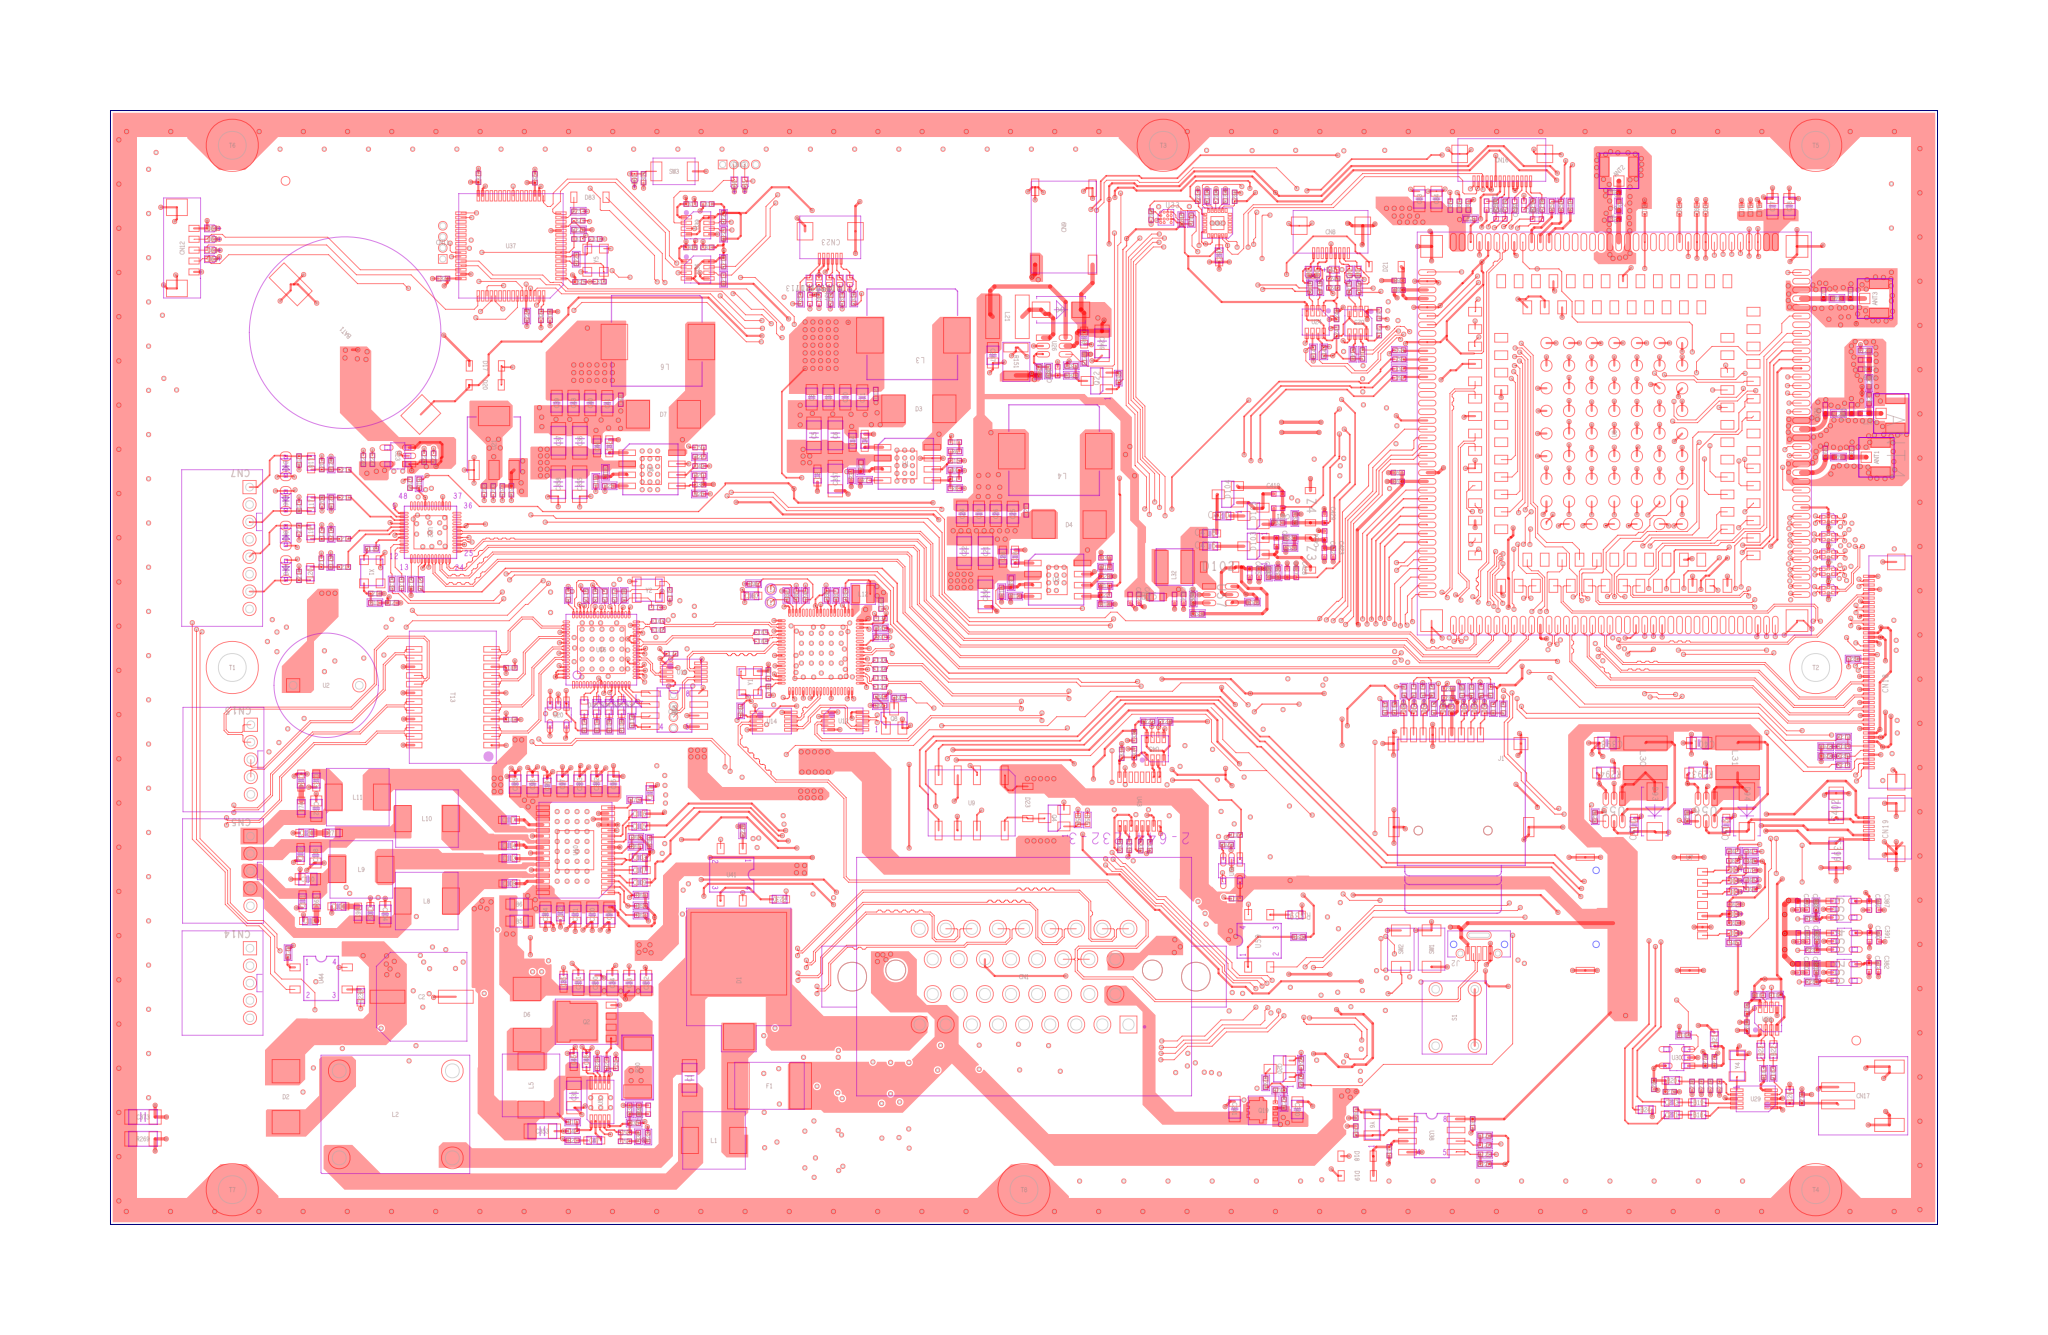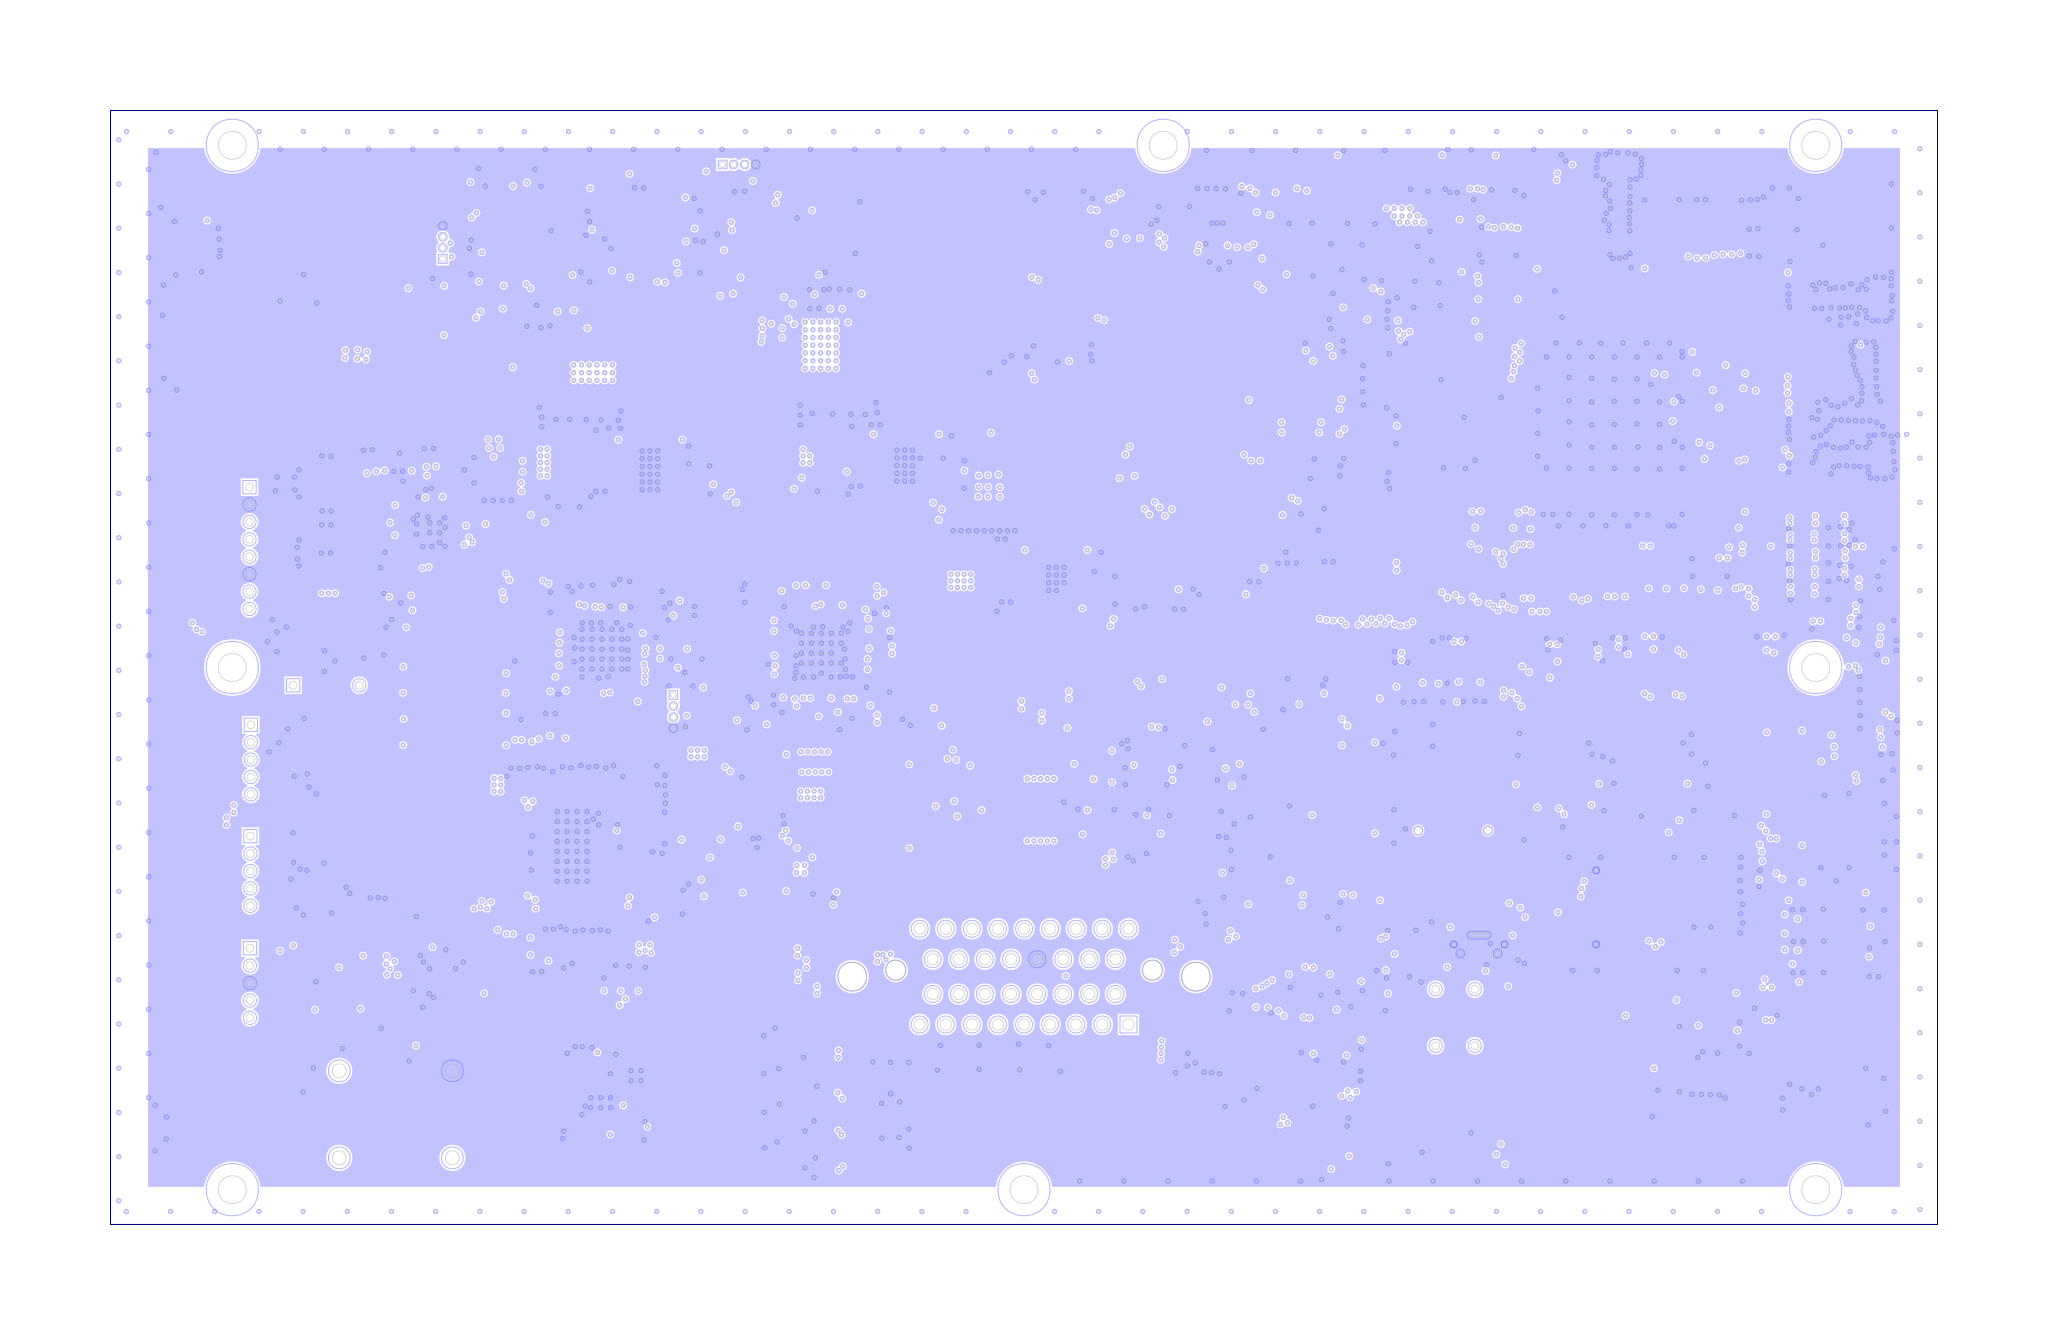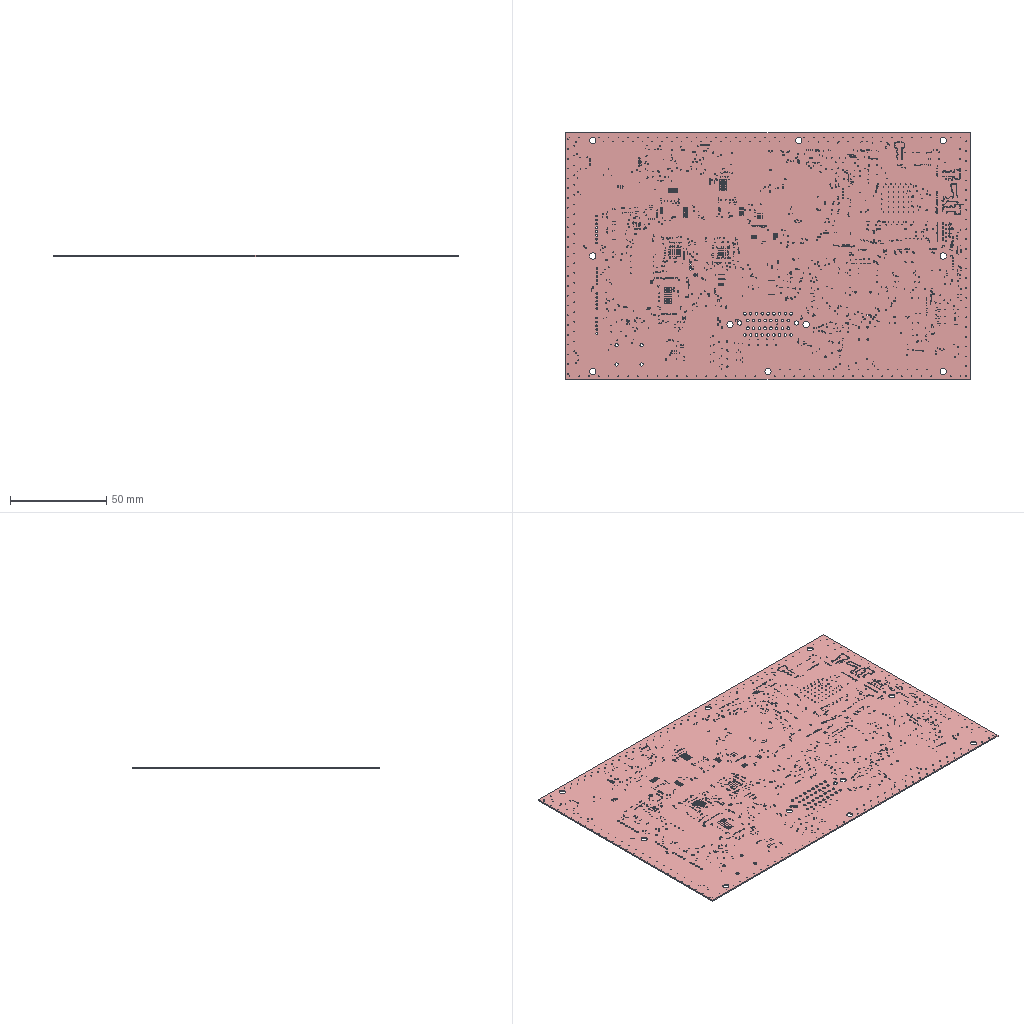Circuit board layout | Cadence Allegro | box 210 x 128 x 0.7 mm
Layer stack:
# Cadence Allegro layer stack of  (unit mm; from the constraint file cross-section; dielectric type: 0 not recorded (Allegro does not mark core vs prepreg), 3 surface material)
index,name,kind,layer,copper_thickness_mm,dielectric_type,dielectric_thickness_mm,dielectric_material,dielectric_constant
0,Top Surface,other,,,,,,
1,TOP,copper,TOP,0.0305,,,,
2,Dielectric1,dielectric,,,0,0.2032,FR-4,4.5
3,L2-GND1,copper,L2-GND1,0.0305,,,,
4,Dielectric2,dielectric,,,0,0.2032,FR-4,4.5
5,L3-PWR,copper,L3-PWR,0.0305,,,,
6,Dielectric3,dielectric,,,0,0.2032,FR-4,4.5
7,BOTTOM,copper,BOTTOM,0.0305,,,,
8,Bottom Surface,other,,,,,,
# drill layer pairs: low layer,high layer
drill_pair,TOP,BOTTOM
Part placement, first 540 of 973 lines:
REFDES,COMP_VALUE,SYM_NAME,SYM_X,SYM_Y,SYM_ROTATE,SYM_MIRROR
ANT1,U.FL-R-SMT-1(80),IPEX,8036.000,5758.000,270.000,NO
ANT2,U.FL-R-SMT-1(80),IPEX,6851.586,7071.978,0.000,NO
ANT3,U.FL-R-SMT-1(80),IPEX,8029.000,6476.000,270.000,NO
ANT4,U.FL-R-SMT-1(80),IPEX,8103.000,5956.000,270.000,NO
B1,120R@100MHz,R0402,6380.000,6896.000,90.000,NO
B2,120R@100MHz,R0402,5858.000,6201.000,180.000,NO
B3,120R@100MHz,R0402,5858.000,6158.000,180.000,NO
B4,120R@100MHz,R0402,5858.000,6117.000,180.000,NO
B5,600R@100MHz,R0805,1875.000,3659.000,0.000,NO
B6,600R@100MHz,R0805,1875.000,3736.000,0.000,NO
B7,120R@100MHz,R0402,2492.000,4867.000,0.000,YES
B8,120R@100MHz,R0402,2474.000,5050.000,0.000,YES
B9,120R@100MHz,R0402,2197.000,5205.000,0.000,YES
B10,120R@100MHz,R0402,2196.000,5113.000,0.000,YES
B11,120R@100MHz,R0402,1223.000,5099.000,180.000,NO
B12,120R@100MHz,R0402,1368.000,5588.000,0.000,YES
B13,120R@100MHz,R0402,1266.000,5652.000,90.000,YES
B14,120R@100MHz,R0402,1518.000,5656.000,90.000,YES
B15,120R@100MHz,R0402,1423.000,5638.000,270.000,NO
B18,1K@100MHz,R0603,7211.000,2783.000,180.000,NO
B19,1K@100MHz,R0603,7212.000,2839.000,180.000,NO
B20,1K@100MHz,R0603,7092.000,2938.000,180.000,NO
B21,1K@100MHz,R0603,7284.000,3125.000,90.000,NO
B22,1K@100MHz,R0603,7551.000,3073.000,270.000,NO
B23,1K@100MHz,R0603,7494.000,3073.000,270.000,NO
B24,1K@100MHz,R0603,6973.000,2806.000,180.000,NO
B25,120R@100MHz,R0603,4760.000,5125.000,0.000,NO
BAT1,BS-08-B2AA008,CR2032,1073.714,6307.425,135.000,NO
C1,10uF,C1206,2646.000,2950.000,90.000,NO
C2,220uF,ED10,1434.000,3317.000,90.000,NO
C3,0.1uF,C0603,3225.000,5675.000,270.000,NO
C4,0.1uF,C0603,3439.000,5832.000,90.000,NO
C5,10uF,C1206,3209.000,5857.000,90.000,NO
C6,10uF,C1206,3306.000,5857.000,90.000,NO
C7,4.7nF,C0402,3846.000,5659.000,180.000,NO
C8,47uF,C0805,3199.000,6029.000,270.000,NO
C9,47uF,C0805,3275.000,6029.000,270.000,NO
C10,47uF,C0805,3351.000,6029.000,270.000,NO
C11,47uF,C0805,3428.000,6028.000,270.000,NO
C12,0.1uF,C0402,3489.000,6044.000,270.000,NO
C14,0.1uF,C0603,3384.000,5832.000,90.000,NO
C15,4.7nF,C0402,3847.000,5742.000,0.000,NO
C17,4.7nF,C0402,3847.000,5826.000,180.000,NO
C18,0.1uF,C0603,4119.000,5308.000,90.000,NO
C19,47uF,C0805,3956.000,5502.000,270.000,NO
C20,22uF,C0805,959.000,4836.000,180.000,YES
C21,10uF,C1206,3986.000,5333.000,90.000,NO
C22,10uF,C1206,3889.000,5333.000,90.000,NO
C23,4.7nF,C0402,4526.000,5135.000,180.000,NO
C24,47uF,C0805,3880.000,5502.000,270.000,NO
C25,47uF,C0805,4109.000,5501.000,270.000,NO
C26,47uF,C0805,4032.000,5502.000,270.000,NO
C27,0.1uF,C0402,4170.000,5517.000,270.000,NO
C28,0.1uF,C0603,4064.000,5308.000,90.000,NO
C29,4.7nF,C0402,4528.000,5219.000,0.000,NO
C30,4.7nF,C0402,4528.000,5303.000,180.000,NO
C31,10uF,C1206,2123.000,2870.000,270.000,NO
C32,0.1uF,C0603,2283.000,5807.000,90.000,NO
C33,22uF,C0805,2373.000,3379.000,90.000,NO
C34,22uF,C0805,2297.000,3379.000,90.000,NO
C35,0.1uF,C0603,2076.000,3385.000,90.000,NO
C36,10uF,C1206,2150.000,5832.000,90.000,NO
C37,10uF,C1206,2053.000,5832.000,90.000,NO
C38,4.7nF,C0402,2690.000,5634.000,180.000,NO
C39,47uF,C0805,2045.000,6003.000,270.000,NO
C40,47uF,C0805,2197.000,6003.000,270.000,NO
C41,47uF,C0805,2274.000,6002.000,270.000,NO
C42,120pF,C0402,2117.000,2709.000,180.000,NO
C43,47uF,C0805,2121.000,6003.000,270.000,NO
C44,0.1uF,C0402,2335.000,6018.000,270.000,NO
C45,0.1uF,C0603,2122.000,3031.000,90.000,NO
C46,0.1uF,C0603,2228.000,5807.000,90.000,NO
C47,220nF,C0603,2215.000,2667.000,0.000,NO
C48,1uF,C0603,2179.000,3031.000,90.000,NO
C49,4.7nF,C0402,2691.000,5718.000,0.000,NO
C50,4.7nF,C0402,2691.000,5802.000,180.000,NO
C51,100pF,C0402,2313.000,3013.000,90.000,NO
C52,22nF,C0402,2354.000,2663.000,0.000,NO
C53,39pF,C0402,2354.000,2703.000,0.000,NO
C60,0.1uF,C0402,6364.000,3432.000,270.000,YES
C61,0.1uF,C0402,5889.000,3372.000,270.000,YES
C62,0.1uF,C0402,7372.000,3735.000,0.000,NO
C63,10uF,C0402,7371.000,3651.000,0.000,NO
C64,33pF,C0402,7447.000,3803.000,0.000,NO
C65,2.2pF(NC),C0402,7905.000,5778.000,90.000,NO
C66,2.2pF(NC),C0402,7786.000,5778.000,90.000,NO
C67,33pF,C0402,7369.000,3932.000,0.000,NO
C68,2.2pF(NC),C0402,6832.071,6956.083,180.000,NO
C69,2.2pF(NC),C0402,6832.071,6835.083,180.000,NO
C70,2.2pF(NC),C0402,7900.000,6496.000,90.000,NO
C71,2.2pF(NC),C0402,7778.000,6495.000,90.000,NO
C72,33pF,C0402,7447.000,3889.000,0.000,NO
C73,0.1uF,C0402,5767.000,3388.000,270.000,YES
C74,33pF,C0402,7407.000,6878.000,90.000,NO
C75,10pF,C0402,7447.000,6878.000,90.000,NO
C76,0.1uF,C0402,7487.000,6878.000,90.000,NO
C77,47uF,C0805,7547.000,6893.000,90.000,NO
C78,47uF,C0805,7623.000,6893.000,90.000,NO
C79,10uF,C0402,6968.000,6878.000,90.000,NO
C80,10uF,C0402,7244.000,6878.000,90.000,NO
C81,10uF,C0402,7204.000,6878.000,90.000,NO
C82,10uF,C0402,7125.000,6878.000,90.000,NO
C83,47uF,C0805,5949.000,6926.000,90.000,NO
C84,47uF,C0805,6026.000,6926.000,90.000,NO
C85,0.1uF,C0402,6089.000,6896.000,90.000,NO
C86,10pF,C0402,6130.000,6896.000,90.000,NO
C87,33pF,C0402,6170.000,6896.000,90.000,NO
C88,10uF,C0402,5855.000,6557.000,180.000,NO
C89,0.1uF,C0402,5855.000,6514.000,180.000,NO
C90,10uF,C0402,5851.000,5648.000,180.000,NO
C91,0.1uF,C0402,5851.000,5688.000,180.000,NO
C95,22uF,C0805,2302.000,4279.000,90.000,NO
C96,22uF,C0805,2283.000,3688.000,270.000,NO
C97,22uF,C0805,2071.000,4279.000,90.000,NO
C98,22uF,C0805,1936.000,4278.000,90.000,NO
C99,0.1uF,C0603,2002.000,4272.000,90.000,NO
C100,22uF,C0805,2206.000,3689.000,270.000,NO
C101,22uF,C0805,2129.000,3689.000,270.000,NO
C102,0.1uF,C0603,2062.000,3694.000,270.000,NO
C103,1uF,C0603,2421.000,3947.000,0.000,NO
C104,680nF,C0805,1269.000,3690.000,90.000,NO
C105,1nF,C0603,1202.000,3696.000,90.000,NO
C106,10nF,C0603,1057.000,3726.000,0.000,NO
C107,1uF,C0603,2421.000,3890.000,180.000,NO
C108,220nF,C0603,1831.000,3829.000,180.000,NO
C109,1uF,C0603,2421.000,3834.000,180.000,NO
C110,680nF,C0805,919.000,3849.000,180.000,NO
C111,1nF,C0603,895.000,3749.000,270.000,NO
C112,10nF,C0603,929.000,3660.000,0.000,NO
C113,220nF,C0603,1831.000,3944.000,180.000,NO
C114,220nF,C0603,1830.000,4001.000,180.000,NO
C115,1uF,C0603,2419.000,4088.000,180.000,NO
C116,1uF,C0603,2420.000,4145.000,180.000,NO
C117,220nF,C0603,1829.000,4117.000,180.000,NO
C118,680nF,C0805,954.000,3957.000,270.000,NO
C119,1nF,C0603,886.000,3963.000,270.000,NO
C120,10nF,C0603,912.000,4058.000,0.000,NO
C121,1uF,C0603,2467.000,4238.000,270.000,NO
C122,680nF,C0805,957.000,4168.000,90.000,NO
C123,1nF,C0603,957.000,4295.000,270.000,NO
C124,10nF,C0603,889.000,4295.000,270.000,NO
C125,22uF,C0805,2463.000,4230.000,180.000,YES
C126,22uF,C0805,2463.000,4318.000,180.000,YES
C127,22uF,C0805,2463.000,4152.000,180.000,YES
C128,1uF,C0603,2347.000,4027.000,0.000,YES
C129,0.1uF,C0402,1515.000,3555.000,90.000,YES
C130,0.1uF,C0402,3362.000,4605.000,180.000,YES
C131,10uF,C0402,3510.000,5028.000,180.000,NO
C132,10uF,C0402,3407.000,5028.000,0.000,YES
C133,0.1uF,C0402,3507.000,4840.000,180.000,NO
C134,0.1uF,C0402,3507.000,4799.000,180.000,NO
C135,0.1uF,C0402,3508.000,4759.000,180.000,NO
C136,0.1uF,C0402,2985.000,4631.000,180.000,YES
C137,0.1uF,C0402,3508.000,4719.000,180.000,NO
C138,18pF,C0402,3003.000,4776.000,90.000,NO
C139,18pF,C0402,3003.000,4701.000,270.000,NO
C140,10uF,C0402,3411.000,4715.000,270.000,YES
C141,10uF,C0402,3329.000,4715.000,270.000,YES
C142,0.1uF,C0402,3513.000,5091.000,270.000,NO
C143,0.1uF,C0402,3402.000,4798.000,0.000,YES
C144,0.1uF,C0402,3287.000,4715.000,270.000,YES
C145,0.1uF,C0402,3161.000,4715.000,270.000,YES
C146,0.1uF,C0402,3086.000,4774.000,180.000,YES
C147,0.1uF,C0402,3086.000,4861.000,180.000,YES
C148,0.1uF,C0402,3086.000,4971.000,180.000,YES
C149,0.1uF,C0402,3086.000,5019.000,180.000,YES
C150,0.1uF,C0402,3249.000,5036.000,90.000,YES
C151,0.1uF,C0402,3402.000,4890.000,0.000,YES
C152,0.1uF,C0402,3370.000,4715.000,270.000,YES
C153,0.1uF,C0402,3402.000,4845.000,0.000,YES
C154,0.1uF,C0402,3208.000,4715.000,270.000,YES
C155,0.1uF,C0402,3114.000,4715.000,270.000,YES
C156,0.1uF,C0402,3086.000,4814.000,180.000,YES
C157,0.1uF,C0402,3207.000,5036.000,90.000,YES
C158,0.1uF,C0402,3407.000,4987.000,0.000,YES
C159,0.1uF,C0402,3351.000,5036.000,90.000,YES
C160,1uF,C0603,2926.000,5131.000,180.000,NO
C161,1nF,C1206,957.000,4414.000,180.000,YES
C162,10uF,C0402,1836.000,4805.000,0.000,NO
C163,0.1uF,C0402,1836.000,4571.000,0.000,NO
C164,1nF,C1206,1158.000,4415.000,0.000,YES
C165,0.1uF,C0402,2970.000,4966.000,0.000,NO
C166,0.1uF,C0402,2505.000,4976.000,0.000,NO
C167,0.1uF,C0402,2504.000,5017.000,0.000,NO
C168,0.1uF,C0402,2970.000,4925.000,0.000,NO
C169,0.1uF,C0402,2685.000,4672.000,0.000,YES
C170,15pF,C0402,2557.000,5138.000,90.000,NO
C171,15pF,C0402,2492.000,5078.000,180.000,NO
C172,0.1uF,C0402,2563.000,4869.000,0.000,NO
C173,0.1uF,C0402,2492.000,4738.000,180.000,YES
C174,10uF,C0402,2079.000,4578.000,270.000,YES
C175,10uF,C0402,2078.000,4658.000,90.000,YES
C176,0.1uF,C0402,2264.000,5028.000,90.000,YES
C177,0.1uF,C0402,2298.000,4738.000,270.000,YES
C178,0.1uF,C0402,2341.000,5028.000,90.000,YES
C179,0.1uF,C0402,2110.000,4918.000,180.000,YES
C180,0.1uF,C0402,2141.000,5028.000,90.000,YES
C181,0.1uF,C0402,2474.000,4966.000,180.000,YES
C182,0.1uF,C0402,2474.000,5007.000,180.000,YES
C183,10uF,C0402,2386.000,4824.000,0.000,YES
C184,0.1uF,C0402,2386.000,4865.000,0.000,YES
C185,10uF,C0402,2386.000,4964.000,0.000,YES
C186,0.1uF,C0402,2386.000,4906.000,0.000,YES
C187,0.1uF,C0402,2386.000,4776.000,0.000,YES
C188,0.1uF,C0402,2257.000,4738.000,270.000,YES
C189,0.1uF,C0402,2223.000,5028.000,90.000,YES
C190,0.1uF,C0402,2110.000,4806.000,180.000,YES
C191,0.1uF,C0402,2182.000,5028.000,90.000,YES
C192,0.1uF,C0402,2110.000,4966.000,180.000,YES
C193,0.1uF,C0402,2110.000,4871.000,180.000,YES
C194,10uF,C0402,2284.000,5163.000,180.000,YES
C195,0.1uF,C0402,2284.000,5205.000,180.000,YES
C196,10uF,C0402,2037.000,5119.000,0.000,YES
C197,0.1uF,C0402,2037.000,5078.000,0.000,YES
C198,10uF,C0402,2622.000,5083.000,180.000,YES
C199,0.1uF,C0402,2622.000,5042.000,180.000,YES
C200,10uF,C0402,2196.000,5155.000,180.000,YES
C201,0.1uF,C0402,2117.000,5120.000,0.000,YES
C202,10uF,C0402,1717.000,5608.000,270.000,NO
C203,0.1uF,C0402,1758.000,5608.000,270.000,NO
C204,10uF,C0402,1840.000,5608.000,270.000,NO
C205,0.1uF,C0402,1799.000,5608.000,270.000,NO
C206,180pF,C0402,879.000,5743.000,270.000,NO
C207,180pF,C0402,982.000,5722.000,90.000,NO
C208,180pF,C0402,879.000,5534.000,90.000,NO
C209,180pF,C0402,983.000,5556.000,270.000,NO
C210,0.1uF,C0402,1084.000,5575.000,0.000,NO
C211,0.1uF,C0402,1084.000,5701.000,0.000,NO
C212,180pF,C0402,879.000,5429.000,270.000,NO
C213,180pF,C0402,982.000,5408.000,90.000,NO
C214,0.1uF,C0402,1082.000,5389.000,0.000,NO
C215,0.1uF,C0402,1082.000,5261.000,0.000,NO
C216,180pF,C0402,879.000,5221.000,90.000,NO
C217,180pF,C0402,980.000,5281.000,90.000,NO
C218,0.1uF,C0402,1223.000,5141.000,0.000,NO
C219,0.1uF,C0402,1300.000,5099.000,0.000,NO
C220,0.1uF,C0402,1368.000,5672.000,0.000,YES
C221,10uF,C0402,1368.000,5630.000,0.000,YES
C222,0.1uF,C0402,1368.000,5546.000,180.000,YES
C223,10uF,C0402,1368.000,5505.000,180.000,YES
C224,0.1uF,C0402,1445.000,5756.000,90.000,NO
C225,10uF,C0402,1488.000,5756.000,90.000,NO
C226,0.1uF,C0402,1170.000,5746.000,90.000,NO
C227,10uF,C0402,1211.000,5746.000,90.000,NO
C228,0.1uF,C0402,1368.000,5410.000,180.000,YES
C229,22uF,C0805,814.000,4924.000,0.000,YES
C230,10uF,C0402,1308.000,5652.000,270.000,YES
C231,22uF,C0805,822.000,5058.000,90.000,YES
C232,0.1uF,C0402,1529.000,5525.000,90.000,YES
C233,0.1uF,C0402,1480.000,5311.000,270.000,YES
C234,0.1uF,C0402,1437.000,5655.000,90.000,YES
C235,10uF,C0402,1478.000,5655.000,90.000,YES
C236,0.1uF,C0402,1580.000,5440.000,0.000,YES
C237,0.1uF,C0402,1580.000,5355.000,0.000,YES
C238,0.1uF,C0402,1450.000,5525.000,90.000,YES
C239,0.1uF,C0402,1439.000,5311.000,270.000,YES
C240,0.1uF,C0402,1381.000,5638.000,90.000,NO
C241,0.1uF,C0402,5574.000,6325.000,90.000,NO
C242,0.1uF,C0402,5574.000,6401.000,270.000,NO
C244,0.1uF,C0402,5559.000,6566.000,180.000,NO
C245,10uF,C0402,5559.000,6524.000,180.000,NO
C247,47uF,C0805,4019.000,6219.000,270.000,NO
C248,1uF,C0603,4432.000,6299.000,270.000,NO
C249,10uF,C1206,4513.000,6273.000,270.000,NO
C268,0.1uF,C0402,7431.000,3260.000,270.000,NO
C269,0.1uF,C0402,7431.000,3182.000,90.000,NO
C270,22pF,C0402,7680.000,2855.000,90.000,NO
C271,1uF,C0603,7091.000,2783.000,180.000,NO
C272,10uF,C0402,7284.000,3025.000,90.000,NO
C273,1uF,C0603,7091.000,2839.000,180.000,NO
C274,0.1uF,C0402,7243.000,3025.000,90.000,NO
C275,0.1uF,C0402,7225.000,2914.000,270.000,NO
C276,10uF,C0402,7183.000,2914.000,270.000,NO
C277,10pF,C0402,7307.000,2914.000,270.000,NO
C278,2.2nF,C0402,7266.000,2914.000,270.000,NO
C279,0.1uF,C0402,7082.000,2887.000,0.000,NO
C280,10uF,C0402,7010.000,2918.000,270.000,NO
C284,10uF,C0402,6080.000,4711.000,0.000,NO
C285,0.1uF,C0402,6080.000,4669.000,0.000,NO
C286,0.1uF,C0402,5113.000,6936.000,90.000,NO
C287,0.1uF,C0402,4946.000,6936.000,90.000,NO
C288,0.1uF,C0402,5029.000,6936.000,90.000,NO
C289,10uF,C0402,4735.000,6851.000,90.000,NO
C290,1uF,C0603,5043.000,6671.000,270.000,NO
C291,10uF,C1206,5149.000,3232.000,270.000,YES
C292,0.1uF,C0603,5229.000,3207.000,270.000,YES
C293,0.1uF,C0402,5541.000,3357.000,90.000,YES
C294,0.1uF,C0402,5542.000,3280.000,270.000,YES
C295,10uF,C1206,5722.000,3236.000,270.000,YES
C296,0.1uF,C0603,5644.000,3211.000,270.000,YES
C297,4.7nF,C0603,4975.000,3048.000,90.000,YES
C298,4.7nF,C0603,5044.000,2901.000,270.000,YES
C299,22uF,C0805,3246.000,2870.000,0.000,YES
C300,22uF,C0805,3597.000,2917.000,90.000,YES
C301,22uF,C0805,3244.000,2709.000,0.000,YES
C302,22uF,C0805,3594.000,2754.000,90.000,YES
C303,22uF,C0805,3245.000,2543.000,0.000,YES
C304,22uF,C0805,3245.000,3062.000,0.000,YES
C305,22uF,C0805,3595.000,2597.000,270.000,YES
C306,22uF,C0805,3597.000,3055.000,90.000,YES
C307,0.1uF,C0402,2727.000,6707.000,180.000,NO
C308,0.1uF,C0402,2650.000,6707.000,0.000,NO
C309,0.1uF,C0402,2438.000,7020.000,270.000,NO
C310,0.1uF,C0402,2727.000,6903.000,180.000,NO
C311,0.1uF,C0402,2651.000,6903.000,0.000,NO
C312,0.1uF,C0402,5813.000,2618.000,270.000,NO
C313,0.1uF,C0402,6190.000,2744.000,270.000,NO
C314,18pF,C0402,2239.000,6552.000,180.000,NO
C315,0.1uF,C0402,5767.000,6328.000,90.000,NO
C316,18pF,C0402,2220.000,6745.000,0.000,NO
C317,0.1uF,C0402,2143.000,6745.000,0.000,NO
C318,100pF,C0402,2914.000,4004.000,180.000,YES
C319,10uF,C0402,2015.000,6397.000,270.000,NO
C320,0.1uF,C0402,1974.000,6397.000,270.000,NO
C321,0.1uF,C0402,2143.000,6828.000,0.000,NO
C322,0.1uF,C0402,1946.414,7019.828,90.000,NO
C323,0.1uF,C0402,1691.000,7022.000,90.000,NO
C324,0.1uF,C0402,1531.000,6566.000,180.000,NO
C325,0.1uF,C0402,2148.000,6551.000,0.000,NO
C326,100pF,C0402,2990.000,4004.000,0.000,YES
C327,10uF,C0402,2953.000,4580.000,0.000,YES
C328,0.1uF,C0402,2953.000,4539.000,0.000,YES
C329,10uF,C0402,1977.000,3370.000,270.000,YES
C330,0.1uF,C0402,1936.000,3370.000,270.000,YES
C331,0.1uF,C0402,4594.000,3999.000,270.000,NO
C332,0.1uF,C0402,4688.000,3998.000,90.000,NO
C333,0.1uF,C0402,4602.000,4416.000,270.000,NO
C334,0.1uF,C0402,4729.000,3998.000,90.000,NO
C335,0.1uF,C0402,4636.000,3999.000,90.000,NO
C336,0.1uF,C0402,4659.000,4496.000,270.000,NO
C337,0.1uF,C0402,4659.000,4419.000,90.000,NO
C338,100pF,C0402,1444.000,3413.000,270.000,YES
C339,100pF,C0402,1444.000,3336.000,90.000,YES
C340,22uF,C0805,5397.000,2807.000,90.000,NO
C341,22uF,C0805,5113.000,2809.000,90.000,NO
C342,0.1uF,C0402,1377.000,3076.000,90.000,YES
C343,0.1uF,C0402,5492.000,4782.000,90.000,YES
C344,0.1uF,C0402,5492.000,4707.000,270.000,YES
C350,22uF,C0805,2220.000,3379.000,90.000,NO
C351,22uF,C0805,2143.000,3380.000,90.000,NO
C352,22uF,C0805,2450.000,3379.000,90.000,NO
C353,10uF,C1206,1980.000,2709.000,0.000,NO
C355,10uF,C1206,2149.000,5636.000,270.000,NO
C356,10uF,C1206,3985.000,5137.000,270.000,NO
C357,10uF,C1206,3306.000,5661.000,270.000,NO
C358,10uF,C1206,2052.000,5636.000,270.000,NO
C361,0.1uF,C0402,1368.000,5457.000,180.000,YES
C362,22uF,C0805,2225.000,4280.000,90.000,NO
C363,22uF,C0805,2149.000,4279.000,90.000,NO
C364,22uF,C0805,1994.000,3689.000,270.000,NO
C365,22uF,C0805,1857.000,4279.000,90.000,NO
C368,10pF,C0402,5661.000,2788.000,90.000,NO
C369,10pF,C0402,5661.000,2712.000,270.000,NO
C370,0.1uF,C0402,5767.000,6405.000,270.000,NO
C371,10uF,C0402,5118.000,3761.000,180.000,NO
C372,10uF,C0402,5118.000,4049.000,180.000,NO
C373,1nF,C1206,173.000,2773.000,180.000,NO
C374,100pF,C0402,2459.000,2806.000,90.000,NO
C375,2.2pF(NC),C0402,7905.000,5975.000,90.000,NO
C376,2.2pF(NC),C0402,7786.000,5975.000,90.000,NO
C377,100pF,C0402,7964.000,5956.000,180.000,NO
C378,0.1uF,C0402,7965.000,6198.000,180.000,NO
C379,1uF,C0402,7965.000,6156.000,180.000,NO
C380,0.1uF,C0402,7662.000,3446.000,270.000,NO
C381,10uF,C0402,7703.000,3446.000,270.000,NO
C382,0.1uF,C0402,8026.000,3450.000,270.000,NO
C383,10uF,C0402,7984.000,3450.000,270.000,NO
C384,0.1uF,C0402,7664.000,3586.000,270.000,NO
C385,10uF,C0402,7705.000,3586.000,270.000,NO
C386,0.1uF,C0402,7985.000,3729.000,270.000,NO
C387,10uF,C0402,8027.000,3729.000,270.000,NO
C388,0.1uF,C0402,7703.000,3730.000,270.000,NO
C389,10uF,C0402,7662.000,3730.000,270.000,NO
C390,0.1uF,C0402,7986.000,3586.000,270.000,NO
C391,10uF,C0402,8029.000,3586.000,270.000,NO
C392,0.1uF,C0402,8092.000,4447.000,180.000,YES
C393,0.1uF,C0402,8092.000,4531.000,180.000,YES
C394,0.1uF,C0402,8087.000,4949.000,180.000,YES
C395,0.1uF,C0402,8087.000,4908.000,180.000,YES
C396,0.1uF,C0402,8087.000,4990.000,180.000,YES
C397,0.1uF,C0402,8092.000,4490.000,180.000,YES
C398,47uF,C0805,6798.000,4465.000,180.000,NO
C399,10uF,C1206,7835.000,3956.000,270.000,NO
C400,1uF,C0603,6921.000,4095.000,90.000,NO
C401,47uF,C0805,7215.000,4465.000,180.000,NO
C402,10uF,C1206,7835.000,4183.000,90.000,NO
C403,1uF,C0603,7338.000,4095.000,90.000,NO
C404,33pF,C0402,6316.000,6836.000,0.000,NO
C405,33pF,C0402,6253.000,6896.000,270.000,NO
C406,33pF,C0402,6481.000,6835.000,0.000,NO
C407,33pF,C0402,6422.000,6897.000,90.000,NO
C408,10uF,C0402,5759.000,6461.000,180.000,YES
C409,0.1uF,C0402,5759.000,6420.000,180.000,YES
C412,0.1uF,C0402,4640.000,5117.000,270.000,NO
C413,10uF,C0402,4679.000,5117.000,270.000,NO
C414,0.1uF,C0402,4841.000,5117.000,270.000,NO
C415,10uF,C0402,4882.000,5117.000,270.000,NO
C416,1uF,C0603,5002.000,5355.000,0.000,NO
C417,0.1uF,C0402,5302.000,5373.000,270.000,NO
C418,1uF,C0603,5002.000,5413.000,0.000,NO
C419,0.1uF,C0402,5310.000,5592.000,0.000,NO
C420,1uF,C0603,5062.000,5492.000,0.000,NO
C421,0.1uF,C0402,5310.000,5527.000,180.000,NO
C422,0.1uF,C0402,5519.000,5326.000,270.000,NO
C423,1uF,C0402,5559.000,5326.000,270.000,NO
C424,1uF,C0402,5520.000,5404.000,90.000,NO
C425,0.1uF,C0402,5181.000,5234.000,270.000,NO
C426,1uF,C0402,5223.000,5234.000,270.000,NO
C427,0.1uF,C0402,5351.000,5234.000,270.000,NO
C428,10uF,C0402,5392.000,5234.000,270.000,NO
C429,1uF,C0402,5520.000,5481.000,270.000,NO
C430,0.1uF,C0402,5131.000,4291.000,270.000,YES
C431,100pF,C0402,5314.000,3950.000,0.000,YES
C432,100pF,C0402,5237.000,3950.000,180.000,YES
C433,100pF,C0402,5284.000,4548.000,0.000,YES
C434,1uF,C0402,4312.000,6147.000,90.000,NO
C435,0.1uF,C0402,5013.000,4482.000,90.000,YES
C436,0.1uF,C0402,3191.000,6472.000,270.000,NO
C437,10uF,C0402,3232.000,6472.000,270.000,NO
CN1,TE_2_6447232_3,TE_2-6447232-3,4160.000,3408.000,180.000,NO
CN5,A2008WR-5P,A2008WR_5P,659.000,3886.000,180.000,NO
CN6,1.27-4P(NC),SIP4_1P27,2573.409,4607.181,270.000,NO
CN7,A2008WR-8P,A2008WR_8P,655.016,5347.000,180.000,NO
CN8,KH-FG0.5-H2.0-9PIN,FPC-9-0P5-2MMH,5549.000,6681.000,180.000,NO
CN9,SM02B-BHSS-1-TB,SM02B,4340.000,6798.000,0.000,NO
CN11,1.27-4P(NC),SIP4_1P27,1529.591,6729.819,90.000,NO
CN12,1.25LT-5P,PH125_5P_SMD_B,404.000,6793.000,270.000,NO
CN13,1.27-4P(NC),SIP4_1P27,2871.000,7082.000,0.000,NO
CN14,A2008WR-5P,A2008WR_5P,657.000,3379.000,180.000,NO
CN15,A2008WR-5P,A2008WR_5P,661.000,4390.000,180.000,NO
CN16,X05A20H14G,FPC-14-0P5-2MMH,6324.000,7006.000,180.000,NO
CN17,PH2.0WT-2P,PH20_2_SMD_B,7961.922,2869.000,270.000,NO
CN18,X05A20H45G,FPC-45-0P5-2MMH,7983.000,4786.000,90.000,NO
CN19,X05A10H06G,FPC-6-0P5-2MMH,7983.000,4078.000,90.000,NO
CN20,X05A20H30G,FPC-30-0P5-2MMH,5652.000,6103.000,270.000,YES
CN23,X05A10H06G,FPC-6-0P5-2MMH,3283.000,6656.000,180.000,NO
CN25,FPC05_10P,FPC-10-0P5-2MMH,5654.000,5516.370,270.000,YES
D1,SM8S33A,DO_218AB,2869.000,3324.000,270.000,NO
D2,MBRS360T3G,SMC,820.000,2865.000,90.000,NO
D3,MBRS360T3G,SMC,3684.000,5977.000,0.000,NO
D4,MBRS360T3G,SMC,4364.000,5453.000,0.000,NO
D5,B5819W,SOD-123,998.000,4924.000,0.000,YES
D6,MBRS360T3G,SMC,1911.000,3237.000,90.000,NO
D7,MBRS360T3G,SMC,2528.000,5952.000,0.000,NO
D8,B5819W,SOD-123,5917.500,3465.000,0.000,YES
D9,TPESD8L3.3CT5G,DFN1006_2L,6404.000,3428.000,0.000,YES
D10,TPESD8L3.3CT5G,DFN1006_2L,5929.000,3368.000,0.000,YES
D11,TPESD8L3.3CT5G,DFN1006_2L,7367.000,3792.000,270.000,NO
D12,TPESD8L3.3CT5G,DFN1006_2L,7366.000,3892.000,270.000,NO
D13,TPESD8L3.3CT5G,DFN1006_2L,7367.000,3692.000,270.000,NO
D14,TPESD8L3.3CT5G,DFN1006_2L,7366.000,3842.000,270.000,NO
D15,TPESD8L3.3CT5G,DFN1006_2L,7367.000,3605.000,270.000,NO
D16,TPESD8L3.3CT5G,DFN1006_2L,5807.000,3368.000,0.000,YES
D17,B5819W,SOD-123,1722.500,6171.000,0.000,NO
D18,B5819W,SOD-123,5667.000,2596.000,0.000,NO
D19,B5819W,SOD-123,5668.000,2507.000,0.000,NO
D20,B5819W,SOD-123,1721.500,6085.000,0.000,NO
D21,B5819W,SOD-123,5794.000,6620.000,0.000,NO
D23,B5819W,SOD-123,4177.000,4196.000,90.000,NO
D26,B5819W,SOD-123,2104.500,3713.000,180.000,YES
D27,B5819W,SOD-123,2035.000,4306.000,180.000,YES
D28,B5819W,SOD-123,2377.000,3881.000,90.000,YES
D29,B5819W,SOD-123,2291.000,3881.000,90.000,YES
D30,B5819W,SOD-123,1654.000,3566.000,0.000,YES
D32,GREEN,D0603,2339.000,4628.000,90.000,NO
D33,YELLOW,D0603,2283.000,4628.000,90.000,NO
D34,RED,D0603,2227.000,4628.000,90.000,NO
D35,GREEN,D0603,2170.000,4627.000,90.000,NO
D36,JEB03CX,SOD-323,819.000,5560.000,270.000,NO
D37,JEB03CX,SOD-323,819.000,5717.000,90.000,NO
D38,JEB03CX,SOD-323,819.000,5403.000,90.000,NO
D39,JEB03CX,SOD-323,820.000,5247.000,270.000,NO
D40,TPESD8L3.3CT5G,DFN1006_2L,5670.000,6595.000,180.000,NO
D41,TPESD8L3.3CT5G,DFN1006_2L,5633.000,6595.000,180.000,NO
D42,TPESD8L3.3CT5G,DFN1006_2L,5559.000,6606.000,90.000,NO
D43,SS34,SMA,4237.000,6425.000,0.000,NO
D44,TPESD8L3.3CT5G,DFN1006_2L,5448.000,6594.000,180.000,NO
D45,TPESD8L3.3CT5G,DFN1006_2L,5486.000,6594.000,180.000,NO
D46,TPESD8L3.3CT5G,DFN1006_2L,5877.000,4616.000,0.000,NO
D47,TPESD8L3.3CT5G,DFN1006_2L,6151.000,4616.000,0.000,NO
D48,TPESD8L3.3CT5G,DFN1006_2L,6056.000,4616.000,0.000,NO
D49,TPESD8L3.3CT5G,DFN1006_2L,6197.000,4616.000,0.000,NO
D50,TPESD8L3.3CT5G,DFN1006_2L,6243.000,4616.000,0.000,NO
D51,TPESD8L3.3CT5G,DFN1006_2L,5925.000,4616.000,0.000,NO
D52,TPESD8L3.3CT5G,DFN1006_2L,5970.000,4616.000,0.000,NO
D53,TPESD8L3.3CT5G,DFN1006_2L,6093.000,4616.000,0.000,NO
D54,MURS260,SMA,5145.000,2898.000,270.000,YES
D55,MURS260,SMA,4846.000,3033.000,90.000,YES
D56,SMAJ12A,SMA,3957.000,3042.000,90.000,YES
D57,SMAJ12A,SMA,4140.000,3042.000,90.000,YES
D58,SMAJ12A,SMA,4324.000,3041.000,90.000,YES
D59,SMAJ12A,SMA,3769.000,3042.000,90.000,YES
D60,TPESD8L3.3CT5G,DFN1006_2L,2397.000,7024.000,180.000,NO
D61,TPESD8L3.3CT5G,DFN1006_2L,479.000,6793.000,270.000,NO
D62,TPESD8L3.3CT5G,DFN1006_2L,479.000,6744.000,270.000,NO
D63,TPESD8L3.3CT5G,DFN1006_2L,479.000,6694.000,270.000,NO
D64,TPESD8L3.3CT5G,DFN1006_2L,479.000,6654.000,270.000,NO
D65,TPESD8L3.3CT5G,DFN1006_2L,2896.000,6998.000,180.000,NO
D66,TPESD8L3.3CT5G,DFN1006_2L,2849.000,6998.000,180.000,NO
D67,PESD2CAN,SOT-23,2952.000,3905.000,0.000,YES
D68,PESD2CAN,SOT-23,953.000,3385.000,270.000,YES
D69,SMAJ12A,SMA,4648.000,4192.000,90.000,YES
D70,SMAJ12A,SMA,4778.000,4191.000,90.000,YES
D73,B5819W,SOD-123,1537.000,3109.000,0.000,YES
D79,TPESD8L3.3CT5G,DFN1006_2L,1598.000,6703.000,270.000,YES
D80,TPESD8L3.3CT5G,DFN1006_2L,1599.000,6740.000,270.000,YES
D83,B5819W,SOD-123,2195.500,6934.000,180.000,NO
D84,B5819W,SOD-123,1537.000,3198.000,0.000,YES
D85,B5819W,SOD-123,1654.000,3653.000,0.000,YES
D86,SMBJ33A,SMB,897.000,3020.000,270.000,YES
D87,SMBJ6.5CA,SMB,2935.000,3745.000,0.000,YES
D88,SMBJ6.5A,SMB,3168.000,3746.000,0.000,YES
D89,SMBJ6.5A,SMB,2702.000,3745.000,180.000,YES
D90,SMBJ6.5CA,SMB,1109.000,3375.000,270.000,YES
D91,SMBJ6.5A,SMB,1306.000,3291.000,0.000,YES
D92,SMBJ6.5A,SMB,1305.000,3459.000,0.000,YES
D93,SS34,SMA,7014.000,4245.000,270.000,NO
D94,SS34,SMA,7431.000,4245.000,270.000,NO
D95,SMBJ33A,SMB,1038.000,3700.000,90.000,YES
D96,TPESD8L3.3CT5G,DFN1006_2L,5755.000,6381.000,270.000,YES
D102,B5819W,SOD-123,5045.000,5261.000,0.000,NO
D103,BAT54S KL4,SOT-23,5198.000,5355.000,90.000,NO
D104,BAT54S KL4,SOT-23,5082.000,5590.000,90.000,NO
D105,BAT54S KL4,SOT-23,5198.000,5492.000,90.000,NO
D106,SMBJ6.5CA,SMB,5260.000,3684.000,0.000,YES
D107,SMBJ6.5A,SMB,5498.000,3683.000,0.000,YES
D108,SMBJ6.5A,SMB,5025.000,3684.000,180.000,YES
D109,PESD2CAN,SOT-23,5269.000,3855.000,0.000,YES
D110,TPESD8L3.3CT5G,DFN1006_2L,3326.000,6554.000,180.000,NO
D111,TPESD8L3.3CT5G,DFN1006_2L,3371.000,6554.000,180.000,NO
D112,TPESD8L3.3CT5G,DFN1006_2L,3278.000,6554.000,180.000,NO
D113,TPESD8L3.3CT5G,DFN1006_2L,3189.000,6554.000,180.000,NO
D114,B5819W,SOD-123,4896.000,4711.000,90.000,YES
D115,SMBJ33A,SMB,4967.000,4099.000,0.000,YES
D116,B5819W,SOD-123,4987.000,4711.000,90.000,YES
D117,TPESD8L3.3CT5G,DFN1006_2L,3232.000,6554.000,180.000,NO
F1,SMD2920P185TS,R2920,3008.000,2914.000,180.000,NO
F2,BSMD0603-001-60V,R0603,4049.000,2892.000,270.000,YES
F3,BSMD0603-001-60V,R0603,4231.000,2892.000,270.000,YES
Pad and via stacks, first 110 of 429 lines:
# Allegro (Cadence) via spans and padstacks; design units: ("mils" 3 1000)
# via spans: padstack,start_layer,end_layer,net_example,count
0503,ETCH/TOP,ETCH/BOTTOM,EGND,2319
# Allegro padstack definitions: name,start_layer,end_layer,drill,plating,holeType,type
PAD1,"ETCH/TOP","ETCH/TOP",0.0,"NON_PLATED","none","smd"
PAD49,"ETCH/TOP","ETCH/TOP",0.0,"NON_PLATED","none","smd"
PAD28,"ETCH/TOP","ETCH/TOP",0.0,"NON_PLATED","none","smd"
PAD16,"ETCH/TOP","ETCH/TOP",0.0,"NON_PLATED","none","smd"
PAD17,"ETCH/TOP","ETCH/TOP",0.0,"NON_PLATED","none","smd"
PAD63,"ETCH/TOP","ETCH/TOP",0.0,"NON_PLATED","none","smd"
PAD76,"ETCH/TOP","ETCH/TOP",0.0,"NON_PLATED","none","smd"
PAD77,"ETCH/TOP","ETCH/TOP",0.0,"NON_PLATED","none","smd"
PAD54,"ETCH/TOP","ETCH/TOP",0.0,"NON_PLATED","none","smd"
PAD53,"ETCH/TOP","ETCH/TOP",0.0,"NON_PLATED","none","smd"
PAD55,"ETCH/TOP","ETCH/TOP",0.0,"NON_PLATED","none","smd"
PAD56,"ETCH/TOP","ETCH/TOP",0.0,"NON_PLATED","none","smd"
PAD57,"ETCH/TOP","ETCH/TOP",0.0,"NON_PLATED","none","smd"
PAD64,"ETCH/TOP","ETCH/TOP",0.0,"NON_PLATED","none","smd"
PAD43,"ETCH/TOP","ETCH/TOP",0.0,"NON_PLATED","none","smd"
PAD71,"ETCH/TOP","ETCH/TOP",0.0,"NON_PLATED","none","smd"
PAD14,"ETCH/TOP","ETCH/TOP",0.0,"NON_PLATED","none","smd"
PAD58,"ETCH/TOP","ETCH/TOP",0.0,"NON_PLATED","none","smd"
PAD59,"ETCH/TOP","ETCH/TOP",0.0,"NON_PLATED","none","smd"
PAD65,"ETCH/TOP","ETCH/TOP",0.0,"NON_PLATED","none","smd"
PAD60,"ETCH/TOP","ETCH/TOP",0.0,"NON_PLATED","none","smd"
PAD61,"ETCH/TOP","ETCH/TOP",0.0,"NON_PLATED","none","smd"
PAD62,"ETCH/TOP","ETCH/TOP",0.0,"NON_PLATED","none","smd"
PAD72,"ETCH/TOP","ETCH/TOP",0.0,"NON_PLATED","none","smd"
PAD66,"ETCH/TOP","ETCH/TOP",0.0,"NON_PLATED","none","smd"
PAD23,"ETCH/TOP","ETCH/TOP",0.0,"NON_PLATED","none","smd"
PAD24,"ETCH/TOP","ETCH/TOP",0.0,"NON_PLATED","none","smd"
PAD25,"ETCH/TOP","ETCH/TOP",0.0,"NON_PLATED","none","smd"
PAD4,"ETCH/TOP","ETCH/TOP",0.0,"NON_PLATED","none","smd"
PAD5,"ETCH/TOP","ETCH/TOP",0.0,"NON_PLATED","none","smd"
PAD3,"ETCH/TOP","ETCH/TOP",0.0,"NON_PLATED","none","smd"
PAD6,"ETCH/TOP","ETCH/TOP",0.0,"NON_PLATED","none","smd"
PAD12,"ETCH/TOP","ETCH/TOP",0.0,"NON_PLATED","none","smd"
PAD11,"ETCH/TOP","ETCH/TOP",0.0,"NON_PLATED","none","smd"
PAD26,"ETCH/TOP","ETCH/TOP",0.0,"NON_PLATED","none","smd"
PAD67,"ETCH/TOP","ETCH/TOP",0.0,"NON_PLATED","none","smd"
PAD27,"ETCH/TOP","ETCH/TOP",0.0,"NON_PLATED","none","smd"
PAD75,"ETCH/TOP","ETCH/TOP",0.0,"NON_PLATED","none","smd"
PAD29,"ETCH/TOP","ETCH/TOP",0.0,"NON_PLATED","none","smd"
PAD30,"ETCH/TOP","ETCH/TOP",0.0,"NON_PLATED","none","smd"
PAD34,"ETCH/TOP","ETCH/TOP",0.0,"NON_PLATED","none","smd"
PAD35,"ETCH/TOP","ETCH/TOP",0.0,"NON_PLATED","none","smd"
PAD13,"ETCH/TOP","ETCH/TOP",0.0,"NON_PLATED","none","smd"
PAD36,"ETCH/TOP","ETCH/TOP",0.0,"NON_PLATED","none","smd"
PAD10,"ETCH/TOP","ETCH/TOP",0.0,"NON_PLATED","none","smd"
PAD38,"ETCH/TOP","ETCH/TOP",0.0,"NON_PLATED","none","smd"
PAD37,"ETCH/TOP","ETCH/TOP",0.0,"NON_PLATED","none","smd"
PAD73,"ETCH/TOP","ETCH/TOP",0.0,"NON_PLATED","none","smd"
PAD39,"ETCH/TOP","ETCH/TOP",0.0,"NON_PLATED","none","smd"
PAD40,"ETCH/TOP","ETCH/TOP",0.0,"NON_PLATED","none","smd"
PAD41,"ETCH/TOP","ETCH/TOP",0.0,"NON_PLATED","none","smd"
PAD44,"ETCH/TOP","ETCH/TOP",0.0,"NON_PLATED","none","smd"
PAD68,"ETCH/TOP","ETCH/TOP",0.0,"NON_PLATED","none","smd"
PAD45,"ETCH/TOP","ETCH/TOP",0.0,"NON_PLATED","none","smd"
PAD47,"ETCH/TOP","ETCH/TOP",0.0,"NON_PLATED","none","smd"
PAD48,"ETCH/TOP","ETCH/TOP",0.0,"NON_PLATED","none","smd"
PAD69,"ETCH/TOP","ETCH/TOP",0.0,"NON_PLATED","none","smd"
PAD70,"ETCH/TOP","ETCH/TOP",0.0,"NON_PLATED","none","smd"
PAD50,"ETCH/TOP","ETCH/TOP",0.0,"NON_PLATED","none","smd"
PAD52,"ETCH/TOP","ETCH/TOP",0.0,"NON_PLATED","none","smd"
PAD51,"ETCH/TOP","ETCH/TOP",0.0,"NON_PLATED","none","smd"
PAD15,"ETCH/TOP","ETCH/TOP",0.0,"NON_PLATED","none","smd"
SMD55_47,"ETCH/TOP","ETCH/TOP",0.0,"PLATED","none","smd"
S32,"ETCH/TOP","ETCH/TOP",0.0,"PLATED","none","smd"
O60X110,"ETCH/TOP","ETCH/TOP",0.0,"PLATED","none","smd"
SMD45_65,"ETCH/TOP","ETCH/TOP",0.0,"PLATED","none","smd"
O50X40,"ETCH/TOP","ETCH/TOP",0.0,"PLATED","none","smd"
O40X50,"ETCH/TOP","ETCH/TOP",0.0,"PLATED","none","smd"
SMD150_60,"ETCH/TOP","ETCH/TOP",0.0,"PLATED","none","smd"
O9X30,"ETCH/TOP","ETCH/TOP",0.0,"PLATED","none","smd"
S150-NS,"ETCH/TOP","ETCH/TOP",0.0,"PLATED","none","smd"
R9X30,"ETCH/TOP","ETCH/TOP",0.0,"PLATED","none","smd"
SMD41_87,"ETCH/TOP","ETCH/TOP",0.0,"PLATED","none","smd"
SMD47_47,"ETCH/TOP","ETCH/TOP",0.0,"PLATED","none","smd"
C40-NP,"ETCH/TOP","ETCH/TOP",0.0,"PLATED","none","smd"
SMD1_05,"ETCH/TOP","ETCH/TOP",0.0,"PLATED","none","smd"
SMD06_06,"ETCH/TOP","ETCH/TOP",0.0,"PLATED","none","smd"
SMDR1_05,"ETCH/TOP","ETCH/TOP",0.0,"PLATED","none","smd"
S52,"ETCH/TOP","ETCH/TOP",0.0,"PLATED","none","smd"
SQ24,"ETCH/TOP","ETCH/TOP",0.0,"NON_PLATED","none","smd"
SMDR_0P5_3P0,"ETCH/TOP","ETCH/TOP",0.0,"PLATED","none","smd"
O30X90,"ETCH/TOP","ETCH/TOP",0.0,"PLATED","none","smd"
R30X90,"ETCH/TOP","ETCH/TOP",0.0,"PLATED","none","smd"
R9X37,"ETCH/TOP","ETCH/TOP",0.0,"PLATED","none","smd"
O9X37,"ETCH/TOP","ETCH/TOP",0.0,"PLATED","none","smd"
S150,"ETCH/TOP","ETCH/TOP",0.0,"PLATED","none","smd"
R25X60,"ETCH/TOP","ETCH/TOP",0.0,"PLATED","none","smd"
O25X60,"ETCH/TOP","ETCH/TOP",0.0,"PLATED","none","smd"
RE52_40,"ETCH/TOP","ETCH/TOP",0.0,"NON_PLATED","none","smd"
SQ40,"ETCH/TOP","ETCH/TOP",0.0,"NON_PLATED","none","smd"
O300X120,"ETCH/TOP","ETCH/TOP",0.0,"PLATED","none","smd"
R28X47,"ETCH/TOP","ETCH/TOP",0.0,"PLATED","none","smd"
O90X120,"ETCH/TOP","ETCH/TOP",0.0,"PLATED","none","smd"
SH24,"ETCH/TOP","ETCH/TOP",0.0,"NON_PLATED","none","smd"
O30X20,"ETCH/TOP","ETCH/TOP",0.0,"PLATED","none","smd"
R40X140,"ETCH/TOP","ETCH/TOP",0.0,"PLATED","none","smd"
R0_7X3_0,"ETCH/TOP","ETCH/TOP",0.0,"PLATED","none","smd"
SMD20_40,"ETCH/TOP","ETCH/TOP",0.0,"PLATED","none","smd"
SMD12_70,"ETCH/TOP","ETCH/TOP",0.0,"PLATED","none","smd"
R32X60,"ETCH/TOP","ETCH/TOP",0.0,"PLATED","none","smd"
R58X80,"ETCH/TOP","ETCH/TOP",0.0,"PLATED","none","smd"
R60X110,"ETCH/TOP","ETCH/TOP",0.0,"PLATED","none","smd"
O12X67,"ETCH/TOP","ETCH/TOP",0.0,"PLATED","none","smd"
R12X67,"ETCH/TOP","ETCH/TOP",0.0,"PLATED","none","smd"
R1_5X1_7,"ETCH/TOP","ETCH/TOP",0.0,"PLATED","none","smd"
R1_0X1_2,"ETCH/TOP","ETCH/TOP",0.0,"PLATED","none","smd"
Design rules, without the lines most boards share, first 6 of 94 lines:
# Cadence Allegro design rules of  (from the Constraint Manager export constraints.dcfx, design unit mil; typed fields in mm)
# columns: name | kind | enabled | priority | scope1 | scope2 | descriptor | typed fields (field=value)
# Allegro precedence (priority 1 wins): 1 Region class-to-class, 2 Region class, 3 Region, 4 class-to-class, 5 DiffPair/Bus/NetGroup override, 6 NetClass, 7 constraint set (CSet) default
# per-layer values are written LAYER=value in the descriptor and LAYER:mm in the typed field; a maximum of 0 means no limit set
# --- net classes (and buses / net groups) ---
TF_SD | NetClass | enabled | 6 | no members | All | Net Class (ElectricalCSet=50R) (members: 0) | electricalcset=50R